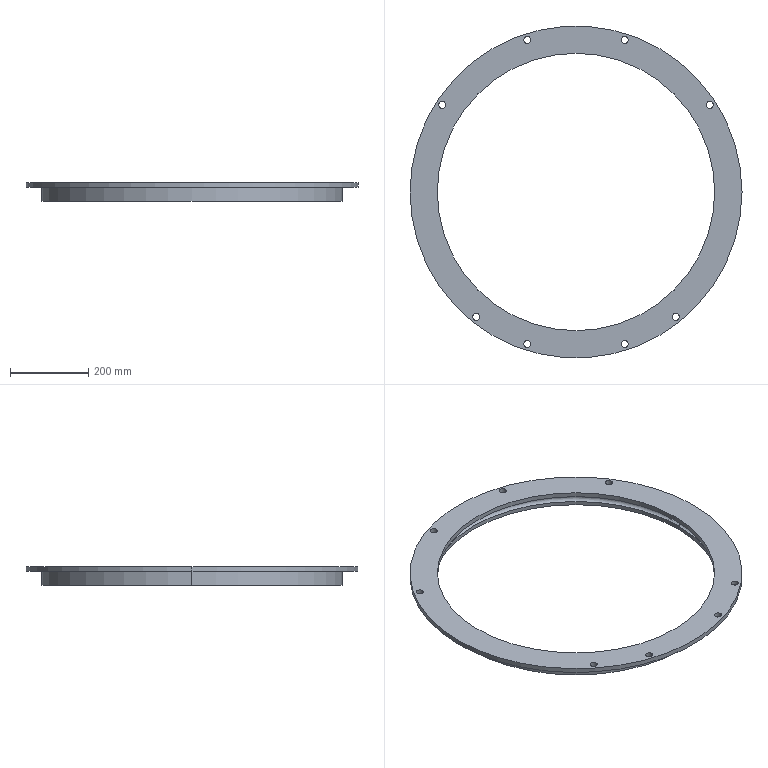Part | SolidWorks | features Cut 1, Extrusion 1, HoleWzd 1, ICE 1, SweepCut 1 | 1 solid | 34 faces | box 850 x 850 x 48 mm | volume 3078442 mm3 | cylinder 28 | plane 4 | torus 2 | commonest cylinder face diameters 18 x16 740 x4 9 x2 710 x2 770 x2 850 x2
STEP:
#1=CARTESIAN_POINT('',(116.,389.43,12.));
#2=VERTEX_POINT('',#1);
#3=CARTESIAN_POINT('',(134.,389.43,12.));
#4=VERTEX_POINT('',#3);
#5=CARTESIAN_POINT('',(125.,389.43,12.));
#6=DIRECTION('',(0.,0.,1.));
#7=DIRECTION('',(1.,0.,0.));
#8=AXIS2_PLACEMENT_3D('',#5,#6,#7);
#9=CIRCLE('',#8,9.);
#10=EDGE_CURVE('',#2,#4,#9,.T.);
#11=ORIENTED_EDGE('',*,*,#10,.T.);
#12=CARTESIAN_POINT('',(134.,389.43,0.));
#13=VERTEX_POINT('',#12);
#14=CARTESIAN_POINT('',(134.,389.43,15.));
#15=DIRECTION('',(0.,0.,-1.));
#16=VECTOR('',#15,1000.);
#17=LINE('',#14,#16);
#18=EDGE_CURVE('',#4,#13,#17,.T.);
#19=ORIENTED_EDGE('',*,*,#18,.T.);
#20=CARTESIAN_POINT('',(116.,389.43,0.));
#21=VERTEX_POINT('',#20);
#22=CARTESIAN_POINT('',(125.,389.43,0.));
#23=DIRECTION('',(0.,0.,-1.));
#24=DIRECTION('',(-1.,0.,0.));
#25=AXIS2_PLACEMENT_3D('',#22,#23,#24);
#26=CIRCLE('',#25,9.);
#27=EDGE_CURVE('',#13,#21,#26,.T.);
#28=ORIENTED_EDGE('',*,*,#27,.T.);
#29=CARTESIAN_POINT('',(116.,389.43,15.));
#30=DIRECTION('',(0.,0.,-1.));
#31=VECTOR('',#30,1000.);
#32=LINE('',#29,#31);
#33=EDGE_CURVE('',#2,#21,#32,.T.);
#34=ORIENTED_EDGE('',*,*,#33,.F.);
#35=EDGE_LOOP('',(#11,#19,#28,#34));
#36=FACE_OUTER_BOUND('',#35,.T.);
#37=CARTESIAN_POINT('',(125.,389.43,15.));
#38=DIRECTION('',(0.,0.,-1.));
#39=DIRECTION('',(-1.,0.,0.));
#40=AXIS2_PLACEMENT_3D('',#37,#38,#39);
#41=CYLINDRICAL_SURFACE('',#40,9.);
#42=ADVANCED_FACE('',(#36),#41,.F.);
#43=CARTESIAN_POINT('',(-264.409,-319.448,12.));
#44=VERTEX_POINT('',#43);
#45=CARTESIAN_POINT('',(-246.409,-319.448,12.));
#46=VERTEX_POINT('',#45);
#47=CARTESIAN_POINT('',(-255.409,-319.448,12.));
#48=DIRECTION('',(0.,0.,1.));
#49=DIRECTION('',(1.,0.,0.));
#50=AXIS2_PLACEMENT_3D('',#47,#48,#49);
#51=CIRCLE('',#50,9.);
#52=EDGE_CURVE('',#44,#46,#51,.T.);
#53=ORIENTED_EDGE('',*,*,#52,.T.);
#54=CARTESIAN_POINT('',(-246.409,-319.448,0.));
#55=VERTEX_POINT('',#54);
#56=CARTESIAN_POINT('',(-246.409,-319.448,15.));
#57=DIRECTION('',(0.,0.,-1.));
#58=VECTOR('',#57,1000.);
#59=LINE('',#56,#58);
#60=EDGE_CURVE('',#46,#55,#59,.T.);
#61=ORIENTED_EDGE('',*,*,#60,.T.);
#62=CARTESIAN_POINT('',(-264.409,-319.448,0.));
#63=VERTEX_POINT('',#62);
#64=CARTESIAN_POINT('',(-255.409,-319.448,0.));
#65=DIRECTION('',(0.,0.,-1.));
#66=DIRECTION('',(-1.,0.,0.));
#67=AXIS2_PLACEMENT_3D('',#64,#65,#66);
#68=CIRCLE('',#67,9.);
#69=EDGE_CURVE('',#55,#63,#68,.T.);
#70=ORIENTED_EDGE('',*,*,#69,.T.);
#71=CARTESIAN_POINT('',(-264.409,-319.448,15.));
#72=DIRECTION('',(0.,0.,-1.));
#73=VECTOR('',#72,1000.);
#74=LINE('',#71,#73);
#75=EDGE_CURVE('',#44,#63,#74,.T.);
#76=ORIENTED_EDGE('',*,*,#75,.F.);
#77=EDGE_LOOP('',(#53,#61,#70,#76));
#78=FACE_OUTER_BOUND('',#77,.T.);
#79=CARTESIAN_POINT('',(-255.409,-319.448,15.));
#80=DIRECTION('',(0.,0.,-1.));
#81=DIRECTION('',(-1.,0.,0.));
#82=AXIS2_PLACEMENT_3D('',#79,#80,#81);
#83=CYLINDRICAL_SURFACE('',#82,9.);
#84=ADVANCED_FACE('',(#78),#83,.F.);
#85=CARTESIAN_POINT('',(246.409,-319.448,12.));
#86=VERTEX_POINT('',#85);
#87=CARTESIAN_POINT('',(264.409,-319.448,12.));
#88=VERTEX_POINT('',#87);
#89=CARTESIAN_POINT('',(255.409,-319.448,12.));
#90=DIRECTION('',(0.,0.,1.));
#91=DIRECTION('',(1.,0.,0.));
#92=AXIS2_PLACEMENT_3D('',#89,#90,#91);
#93=CIRCLE('',#92,9.);
#94=EDGE_CURVE('',#86,#88,#93,.T.);
#95=ORIENTED_EDGE('',*,*,#94,.T.);
#96=CARTESIAN_POINT('',(264.409,-319.448,0.));
#97=VERTEX_POINT('',#96);
#98=CARTESIAN_POINT('',(264.409,-319.448,15.));
#99=DIRECTION('',(0.,0.,-1.));
#100=VECTOR('',#99,1000.);
#101=LINE('',#98,#100);
#102=EDGE_CURVE('',#88,#97,#101,.T.);
#103=ORIENTED_EDGE('',*,*,#102,.T.);
#104=CARTESIAN_POINT('',(246.409,-319.448,0.));
#105=VERTEX_POINT('',#104);
#106=CARTESIAN_POINT('',(255.409,-319.448,0.));
#107=DIRECTION('',(0.,0.,-1.));
#108=DIRECTION('',(-1.,0.,0.));
#109=AXIS2_PLACEMENT_3D('',#106,#107,#108);
#110=CIRCLE('',#109,9.);
#111=EDGE_CURVE('',#97,#105,#110,.T.);
#112=ORIENTED_EDGE('',*,*,#111,.T.);
#113=CARTESIAN_POINT('',(246.409,-319.448,15.));
#114=DIRECTION('',(0.,0.,-1.));
#115=VECTOR('',#114,1000.);
#116=LINE('',#113,#115);
#117=EDGE_CURVE('',#86,#105,#116,.T.);
#118=ORIENTED_EDGE('',*,*,#117,.F.);
#119=EDGE_LOOP('',(#95,#103,#112,#118));
#120=FACE_OUTER_BOUND('',#119,.T.);
#121=CARTESIAN_POINT('',(255.409,-319.448,15.));
#122=DIRECTION('',(0.,0.,-1.));
#123=DIRECTION('',(-1.,0.,0.));
#124=AXIS2_PLACEMENT_3D('',#121,#122,#123);
#125=CYLINDRICAL_SURFACE('',#124,9.);
#126=ADVANCED_FACE('',(#120),#125,.F.);
#127=CARTESIAN_POINT('',(-134.,-389.43,12.));
#128=VERTEX_POINT('',#127);
#129=CARTESIAN_POINT('',(-116.,-389.43,12.));
#130=VERTEX_POINT('',#129);
#131=CARTESIAN_POINT('',(-125.,-389.43,12.));
#132=DIRECTION('',(0.,0.,1.));
#133=DIRECTION('',(1.,0.,0.));
#134=AXIS2_PLACEMENT_3D('',#131,#132,#133);
#135=CIRCLE('',#134,9.);
#136=EDGE_CURVE('',#128,#130,#135,.T.);
#137=ORIENTED_EDGE('',*,*,#136,.T.);
#138=CARTESIAN_POINT('',(-116.,-389.43,0.));
#139=VERTEX_POINT('',#138);
#140=CARTESIAN_POINT('',(-116.,-389.43,15.));
#141=DIRECTION('',(0.,0.,-1.));
#142=VECTOR('',#141,1000.);
#143=LINE('',#140,#142);
#144=EDGE_CURVE('',#130,#139,#143,.T.);
#145=ORIENTED_EDGE('',*,*,#144,.T.);
#146=CARTESIAN_POINT('',(-134.,-389.43,0.));
#147=VERTEX_POINT('',#146);
#148=CARTESIAN_POINT('',(-125.,-389.43,0.));
#149=DIRECTION('',(0.,0.,-1.));
#150=DIRECTION('',(-1.,0.,0.));
#151=AXIS2_PLACEMENT_3D('',#148,#149,#150);
#152=CIRCLE('',#151,9.);
#153=EDGE_CURVE('',#139,#147,#152,.T.);
#154=ORIENTED_EDGE('',*,*,#153,.T.);
#155=CARTESIAN_POINT('',(-134.,-389.43,15.));
#156=DIRECTION('',(0.,0.,-1.));
#157=VECTOR('',#156,1000.);
#158=LINE('',#155,#157);
#159=EDGE_CURVE('',#128,#147,#158,.T.);
#160=ORIENTED_EDGE('',*,*,#159,.F.);
#161=EDGE_LOOP('',(#137,#145,#154,#160));
#162=FACE_OUTER_BOUND('',#161,.T.);
#163=CARTESIAN_POINT('',(-125.,-389.43,15.));
#164=DIRECTION('',(0.,0.,-1.));
#165=DIRECTION('',(-1.,0.,0.));
#166=AXIS2_PLACEMENT_3D('',#163,#164,#165);
#167=CYLINDRICAL_SURFACE('',#166,9.);
#168=ADVANCED_FACE('',(#162),#167,.F.);
#169=CARTESIAN_POINT('',(-134.,389.43,12.));
#170=VERTEX_POINT('',#169);
#171=CARTESIAN_POINT('',(-116.,389.43,12.));
#172=VERTEX_POINT('',#171);
#173=CARTESIAN_POINT('',(-125.,389.43,12.));
#174=DIRECTION('',(0.,0.,1.));
#175=DIRECTION('',(1.,0.,0.));
#176=AXIS2_PLACEMENT_3D('',#173,#174,#175);
#177=CIRCLE('',#176,9.);
#178=EDGE_CURVE('',#170,#172,#177,.T.);
#179=ORIENTED_EDGE('',*,*,#178,.T.);
#180=CARTESIAN_POINT('',(-116.,389.43,0.));
#181=VERTEX_POINT('',#180);
#182=CARTESIAN_POINT('',(-116.,389.43,15.));
#183=DIRECTION('',(0.,0.,-1.));
#184=VECTOR('',#183,1000.);
#185=LINE('',#182,#184);
#186=EDGE_CURVE('',#172,#181,#185,.T.);
#187=ORIENTED_EDGE('',*,*,#186,.T.);
#188=CARTESIAN_POINT('',(-134.,389.43,0.));
#189=VERTEX_POINT('',#188);
#190=CARTESIAN_POINT('',(-125.,389.43,0.));
#191=DIRECTION('',(0.,0.,-1.));
#192=DIRECTION('',(-1.,0.,0.));
#193=AXIS2_PLACEMENT_3D('',#190,#191,#192);
#194=CIRCLE('',#193,9.);
#195=EDGE_CURVE('',#181,#189,#194,.T.);
#196=ORIENTED_EDGE('',*,*,#195,.T.);
#197=CARTESIAN_POINT('',(-134.,389.43,15.));
#198=DIRECTION('',(0.,0.,-1.));
#199=VECTOR('',#198,1000.);
#200=LINE('',#197,#199);
#201=EDGE_CURVE('',#170,#189,#200,.T.);
#202=ORIENTED_EDGE('',*,*,#201,.F.);
#203=EDGE_LOOP('',(#179,#187,#196,#202));
#204=FACE_OUTER_BOUND('',#203,.T.);
#205=CARTESIAN_POINT('',(-125.,389.43,15.));
#206=DIRECTION('',(0.,0.,-1.));
#207=DIRECTION('',(-1.,0.,0.));
#208=AXIS2_PLACEMENT_3D('',#205,#206,#207);
#209=CYLINDRICAL_SURFACE('',#208,9.);
#210=ADVANCED_FACE('',(#204),#209,.F.);
#211=CARTESIAN_POINT('',(-351.768,223.139,12.));
#212=VERTEX_POINT('',#211);
#213=CARTESIAN_POINT('',(-333.768,223.139,12.));
#214=VERTEX_POINT('',#213);
#215=CARTESIAN_POINT('',(-342.768,223.139,12.));
#216=DIRECTION('',(0.,0.,1.));
#217=DIRECTION('',(1.,0.,0.));
#218=AXIS2_PLACEMENT_3D('',#215,#216,#217);
#219=CIRCLE('',#218,9.);
#220=EDGE_CURVE('',#212,#214,#219,.T.);
#221=ORIENTED_EDGE('',*,*,#220,.T.);
#222=CARTESIAN_POINT('',(-333.768,223.139,0.));
#223=VERTEX_POINT('',#222);
#224=CARTESIAN_POINT('',(-333.768,223.139,15.));
#225=DIRECTION('',(0.,0.,-1.));
#226=VECTOR('',#225,1000.);
#227=LINE('',#224,#226);
#228=EDGE_CURVE('',#214,#223,#227,.T.);
#229=ORIENTED_EDGE('',*,*,#228,.T.);
#230=CARTESIAN_POINT('',(-351.768,223.139,0.));
#231=VERTEX_POINT('',#230);
#232=CARTESIAN_POINT('',(-342.768,223.139,0.));
#233=DIRECTION('',(0.,0.,-1.));
#234=DIRECTION('',(-1.,0.,0.));
#235=AXIS2_PLACEMENT_3D('',#232,#233,#234);
#236=CIRCLE('',#235,9.);
#237=EDGE_CURVE('',#223,#231,#236,.T.);
#238=ORIENTED_EDGE('',*,*,#237,.T.);
#239=CARTESIAN_POINT('',(-351.768,223.139,15.));
#240=DIRECTION('',(0.,0.,-1.));
#241=VECTOR('',#240,1000.);
#242=LINE('',#239,#241);
#243=EDGE_CURVE('',#212,#231,#242,.T.);
#244=ORIENTED_EDGE('',*,*,#243,.F.);
#245=EDGE_LOOP('',(#221,#229,#238,#244));
#246=FACE_OUTER_BOUND('',#245,.T.);
#247=CARTESIAN_POINT('',(-342.768,223.139,15.));
#248=DIRECTION('',(0.,0.,-1.));
#249=DIRECTION('',(-1.,0.,0.));
#250=AXIS2_PLACEMENT_3D('',#247,#248,#249);
#251=CYLINDRICAL_SURFACE('',#250,9.);
#252=ADVANCED_FACE('',(#246),#251,.F.);
#253=CARTESIAN_POINT('',(333.768,223.139,12.));
#254=VERTEX_POINT('',#253);
#255=CARTESIAN_POINT('',(351.768,223.139,12.));
#256=VERTEX_POINT('',#255);
#257=CARTESIAN_POINT('',(342.768,223.139,12.));
#258=DIRECTION('',(0.,0.,1.));
#259=DIRECTION('',(1.,0.,0.));
#260=AXIS2_PLACEMENT_3D('',#257,#258,#259);
#261=CIRCLE('',#260,9.);
#262=EDGE_CURVE('',#254,#256,#261,.T.);
#263=ORIENTED_EDGE('',*,*,#262,.T.);
#264=CARTESIAN_POINT('',(351.768,223.139,0.));
#265=VERTEX_POINT('',#264);
#266=CARTESIAN_POINT('',(351.768,223.139,15.));
#267=DIRECTION('',(0.,0.,-1.));
#268=VECTOR('',#267,1000.);
#269=LINE('',#266,#268);
#270=EDGE_CURVE('',#256,#265,#269,.T.);
#271=ORIENTED_EDGE('',*,*,#270,.T.);
#272=CARTESIAN_POINT('',(333.768,223.139,0.));
#273=VERTEX_POINT('',#272);
#274=CARTESIAN_POINT('',(342.768,223.139,0.));
#275=DIRECTION('',(0.,0.,-1.));
#276=DIRECTION('',(-1.,0.,0.));
#277=AXIS2_PLACEMENT_3D('',#274,#275,#276);
#278=CIRCLE('',#277,9.);
#279=EDGE_CURVE('',#265,#273,#278,.T.);
#280=ORIENTED_EDGE('',*,*,#279,.T.);
#281=CARTESIAN_POINT('',(333.768,223.139,15.));
#282=DIRECTION('',(0.,0.,-1.));
#283=VECTOR('',#282,1000.);
#284=LINE('',#281,#283);
#285=EDGE_CURVE('',#254,#273,#284,.T.);
#286=ORIENTED_EDGE('',*,*,#285,.F.);
#287=EDGE_LOOP('',(#263,#271,#280,#286));
#288=FACE_OUTER_BOUND('',#287,.T.);
#289=CARTESIAN_POINT('',(342.768,223.139,15.));
#290=DIRECTION('',(0.,0.,-1.));
#291=DIRECTION('',(-1.,0.,0.));
#292=AXIS2_PLACEMENT_3D('',#289,#290,#291);
#293=CYLINDRICAL_SURFACE('',#292,9.);
#294=ADVANCED_FACE('',(#288),#293,.F.);
#295=CARTESIAN_POINT('',(116.,-389.43,12.));
#296=VERTEX_POINT('',#295);
#297=CARTESIAN_POINT('',(134.,-389.43,12.));
#298=VERTEX_POINT('',#297);
#299=CARTESIAN_POINT('',(125.,-389.43,12.));
#300=DIRECTION('',(0.,0.,1.));
#301=DIRECTION('',(1.,0.,0.));
#302=AXIS2_PLACEMENT_3D('',#299,#300,#301);
#303=CIRCLE('',#302,9.);
#304=EDGE_CURVE('',#296,#298,#303,.T.);
#305=ORIENTED_EDGE('',*,*,#304,.T.);
#306=CARTESIAN_POINT('',(134.,-389.43,0.));
#307=VERTEX_POINT('',#306);
#308=CARTESIAN_POINT('',(134.,-389.43,15.));
#309=DIRECTION('',(0.,0.,-1.));
#310=VECTOR('',#309,1000.);
#311=LINE('',#308,#310);
#312=EDGE_CURVE('',#298,#307,#311,.T.);
#313=ORIENTED_EDGE('',*,*,#312,.T.);
#314=CARTESIAN_POINT('',(116.,-389.43,0.));
#315=VERTEX_POINT('',#314);
#316=CARTESIAN_POINT('',(125.,-389.43,0.));
#317=DIRECTION('',(0.,0.,-1.));
#318=DIRECTION('',(-1.,0.,0.));
#319=AXIS2_PLACEMENT_3D('',#316,#317,#318);
#320=CIRCLE('',#319,9.);
#321=EDGE_CURVE('',#307,#315,#320,.T.);
#322=ORIENTED_EDGE('',*,*,#321,.T.);
#323=CARTESIAN_POINT('',(116.,-389.43,15.));
#324=DIRECTION('',(0.,0.,-1.));
#325=VECTOR('',#324,1000.);
#326=LINE('',#323,#325);
#327=EDGE_CURVE('',#296,#315,#326,.T.);
#328=ORIENTED_EDGE('',*,*,#327,.F.);
#329=EDGE_LOOP('',(#305,#313,#322,#328));
#330=FACE_OUTER_BOUND('',#329,.T.);
#331=CARTESIAN_POINT('',(125.,-389.43,15.));
#332=DIRECTION('',(0.,0.,-1.));
#333=DIRECTION('',(-1.,0.,0.));
#334=AXIS2_PLACEMENT_3D('',#331,#332,#333);
#335=CYLINDRICAL_SURFACE('',#334,9.);
#336=ADVANCED_FACE('',(#330),#335,.F.);
#337=CARTESIAN_POINT('',(385.,0.,-22.5));
#338=VERTEX_POINT('',#337);
#339=CARTESIAN_POINT('',(385.,0.,-13.5));
#340=VERTEX_POINT('',#339);
#341=CARTESIAN_POINT('',(385.,0.,-22.5));
#342=CARTESIAN_POINT('',(385.,-0.2973,-22.5));
#343=CARTESIAN_POINT('',(385.,-0.5897,-22.471));
#344=CARTESIAN_POINT('',(384.998,-1.165,-22.356));
#345=CARTESIAN_POINT('',(384.997,-1.451,-22.27));
#346=CARTESIAN_POINT('',(384.995,-1.996,-22.044));
#347=CARTESIAN_POINT('',(384.993,-2.254,-21.906));
#348=CARTESIAN_POINT('',(384.99,-2.743,-21.579));
#349=CARTESIAN_POINT('',(384.989,-2.975,-21.389));
#350=CARTESIAN_POINT('',(384.985,-3.39,-20.974));
#351=CARTESIAN_POINT('',(384.983,-3.576,-20.747));
#352=CARTESIAN_POINT('',(384.98,-3.905,-20.255));
#353=CARTESIAN_POINT('',(384.979,-4.045,-19.993));
#354=CARTESIAN_POINT('',(384.976,-4.269,-19.452));
#355=CARTESIAN_POINT('',(384.975,-4.356,-19.168));
#356=CARTESIAN_POINT('',(384.974,-4.471,-18.587));
#357=CARTESIAN_POINT('',(384.974,-4.5,-18.295));
#358=CARTESIAN_POINT('',(384.974,-4.5,-17.708));
#359=CARTESIAN_POINT('',(384.974,-4.471,-17.41));
#360=CARTESIAN_POINT('',(384.975,-4.356,-16.833));
#361=CARTESIAN_POINT('',(384.976,-4.271,-16.552));
#362=CARTESIAN_POINT('',(384.979,-4.046,-16.007));
#363=CARTESIAN_POINT('',(384.98,-3.905,-15.744));
#364=CARTESIAN_POINT('',(384.983,-3.579,-15.256));
#365=CARTESIAN_POINT('',(384.985,-3.393,-15.029));
#366=CARTESIAN_POINT('',(384.989,-2.973,-14.609));
#367=CARTESIAN_POINT('',(384.99,-2.745,-14.422));
#368=CARTESIAN_POINT('',(384.993,-2.258,-14.096));
#369=CARTESIAN_POINT('',(384.995,-1.995,-13.955));
#370=CARTESIAN_POINT('',(384.997,-1.449,-13.729));
#371=CARTESIAN_POINT('',(384.998,-1.169,-13.644));
#372=CARTESIAN_POINT('',(385.,-0.592,-13.529));
#373=CARTESIAN_POINT('',(385.,-0.2937,-13.5));
#374=CARTESIAN_POINT('',(385.,0.,-13.5));
#375=B_SPLINE_CURVE_WITH_KNOTS('',3,(#341,#342,#343,#344,#345,#346,#347,#348,#349,#350,#351,#352,#353,#354,#355,#356,#357,#358,#359,#360,#361,#362,#363,#364,#365,#366,#367,#368,#369,#370,#371,#372,#373,#374),.UNSPECIFIED.,.F.,.F.,(4,2,2,2,2,2,2,2,2,2,2,2,2,2,2,2,4),(0.,0.0008793,0.001759,0.002638,0.003517,0.004397,0.005276,0.006155,0.007035,0.007914,0.008793,0.009673,0.01055,0.01143,0.01231,0.01319,0.01407),.UNSPECIFIED.);
#376=EDGE_CURVE('',#338,#340,#375,.T.);
#377=ORIENTED_EDGE('',*,*,#376,.F.);
#378=CARTESIAN_POINT('',(376.614,0.,-22.5));
#379=VERTEX_POINT('',#378);
#380=CARTESIAN_POINT('',(0.,0.,-22.5));
#381=DIRECTION('',(-1.,0.,0.));
#382=VECTOR('',#381,1000.);
#383=LINE('',#380,#382);
#384=EDGE_CURVE('',#338,#379,#383,.T.);
#385=ORIENTED_EDGE('',*,*,#384,.T.);
#386=CARTESIAN_POINT('',(376.614,0.,-13.5));
#387=VERTEX_POINT('',#386);
#388=CARTESIAN_POINT('',(376.614,0.,-13.5));
#389=CARTESIAN_POINT('',(376.614,-0.3013,-13.5));
#390=CARTESIAN_POINT('',(376.635,-0.5988,-13.53));
#391=CARTESIAN_POINT('',(376.712,-1.187,-13.649));
#392=CARTESIAN_POINT('',(376.768,-1.472,-13.738));
#393=CARTESIAN_POINT('',(376.904,-2.013,-13.965));
#394=CARTESIAN_POINT('',(376.984,-2.273,-14.105));
#395=CARTESIAN_POINT('',(377.151,-2.753,-14.428));
#396=CARTESIAN_POINT('',(377.238,-2.975,-14.611));
#397=CARTESIAN_POINT('',(377.413,-3.384,-15.02));
#398=CARTESIAN_POINT('',(377.498,-3.57,-15.245));
#399=CARTESIAN_POINT('',(377.654,-3.893,-15.724));
#400=CARTESIAN_POINT('',(377.724,-4.032,-15.98));
#401=CARTESIAN_POINT('',(377.845,-4.264,-16.53));
#402=CARTESIAN_POINT('',(377.892,-4.351,-16.813));
#403=CARTESIAN_POINT('',(377.94,-4.439,-17.25));
#404=CARTESIAN_POINT('',(377.952,-4.462,-17.397));
#405=CARTESIAN_POINT('',(377.969,-4.492,-17.697));
#406=CARTESIAN_POINT('',(377.973,-4.5,-17.85));
#407=CARTESIAN_POINT('',(377.973,-4.5,-18.303));
#408=CARTESIAN_POINT('',(377.956,-4.47,-18.6));
#409=CARTESIAN_POINT('',(377.908,-4.38,-19.041));
#410=CARTESIAN_POINT('',(377.888,-4.343,-19.188));
#411=CARTESIAN_POINT('',(377.84,-4.255,-19.474));
#412=CARTESIAN_POINT('',(377.814,-4.204,-19.613));
#413=CARTESIAN_POINT('',(377.724,-4.032,-20.02));
#414=CARTESIAN_POINT('',(377.652,-3.89,-20.28));
#415=CARTESIAN_POINT('',(377.495,-3.563,-20.764));
#416=CARTESIAN_POINT('',(377.41,-3.379,-20.986));
#417=CARTESIAN_POINT('',(377.236,-2.969,-21.394));
#418=CARTESIAN_POINT('',(377.147,-2.744,-21.578));
#419=CARTESIAN_POINT('',(376.981,-2.266,-21.899));
#420=CARTESIAN_POINT('',(376.903,-2.011,-22.037));
#421=CARTESIAN_POINT('',(376.767,-1.466,-22.265));
#422=CARTESIAN_POINT('',(376.712,-1.185,-22.351));
#423=CARTESIAN_POINT('',(376.654,-0.7496,-22.44));
#424=CARTESIAN_POINT('',(376.64,-0.6023,-22.462));
#425=CARTESIAN_POINT('',(376.62,-0.3029,-22.492));
#426=CARTESIAN_POINT('',(376.614,-0.1504,-22.5));
#427=CARTESIAN_POINT('',(376.614,0.,-22.5));
#428=B_SPLINE_CURVE_WITH_KNOTS('',3,(#388,#389,#390,#391,#392,#393,#394,#395,#396,#397,#398,#399,#400,#401,#402,#403,#404,#405,#406,#407,#408,#409,#410,#411,#412,#413,#414,#415,#416,#417,#418,#419,#420,#421,#422,#423,#424,#425,#426,#427),.UNSPECIFIED.,.F.,.F.,(4,2,2,2,2,2,2,2,2,2,2,2,2,2,2,2,2,2,2,4),(0.01771,0.01861,0.01951,0.0204,0.0213,0.0222,0.0231,0.02399,0.02444,0.02489,0.02579,0.02624,0.02669,0.02759,0.02848,0.02938,0.03028,0.03118,0.03163,0.03208),.UNSPECIFIED.);
#429=EDGE_CURVE('',#387,#379,#428,.T.);
#430=ORIENTED_EDGE('',*,*,#429,.F.);
#431=CARTESIAN_POINT('',(0.,0.,-13.5));
#432=DIRECTION('',(-1.,0.,0.));
#433=VECTOR('',#432,1000.);
#434=LINE('',#431,#433);
#435=EDGE_CURVE('',#340,#387,#434,.T.);
#436=ORIENTED_EDGE('',*,*,#435,.F.);
#437=EDGE_LOOP('',(#377,#385,#430,#436));
#438=FACE_OUTER_BOUND('',#437,.T.);
#439=CARTESIAN_POINT('',(0.,0.,-18.));
#440=DIRECTION('',(-1.,0.,0.));
#441=DIRECTION('',(0.,0.,1.));
#442=AXIS2_PLACEMENT_3D('',#439,#440,#441);
#443=CYLINDRICAL_SURFACE('',#442,4.5);
#444=ADVANCED_FACE('',(#438),#443,.F.);
#445=CARTESIAN_POINT('',(370.,0.,-26.));
#446=VERTEX_POINT('',#445);
#447=CARTESIAN_POINT('',(-370.,0.,-26.));
#448=VERTEX_POINT('',#447);
#449=CARTESIAN_POINT('',(0.,0.,-26.));
#450=DIRECTION('',(0.,0.,-1.));
#451=DIRECTION('',(1.,0.,0.));
#452=AXIS2_PLACEMENT_3D('',#449,#450,#451);
#453=CIRCLE('',#452,370.);
#454=EDGE_CURVE('',#446,#448,#453,.T.);
#455=ORIENTED_EDGE('',*,*,#454,.T.);
#456=CARTESIAN_POINT('',(-370.,0.,-10.));
#457=VERTEX_POINT('',#456);
#458=CARTESIAN_POINT('',(-370.,0.,-18.));
#459=DIRECTION('',(0.,1.,0.));
#460=DIRECTION('',(-1.,0.,0.));
#461=AXIS2_PLACEMENT_3D('',#458,#459,#460);
#462=CIRCLE('',#461,8.);
#463=EDGE_CURVE('',#448,#457,#462,.T.);
#464=ORIENTED_EDGE('',*,*,#463,.T.);
#465=CARTESIAN_POINT('',(370.,0.,-10.));
#466=VERTEX_POINT('',#465);
#467=CARTESIAN_POINT('',(0.,0.,-10.));
#468=DIRECTION('',(0.,0.,1.));
#469=DIRECTION('',(-1.,0.,0.));
#470=AXIS2_PLACEMENT_3D('',#467,#468,#469);
#471=CIRCLE('',#470,370.);
#472=EDGE_CURVE('',#457,#466,#471,.T.);
#473=ORIENTED_EDGE('',*,*,#472,.T.);
#474=CARTESIAN_POINT('',(370.,0.,-18.));
#475=DIRECTION('',(0.,-1.,0.));
#476=DIRECTION('',(0.,0.,-1.));
#477=AXIS2_PLACEMENT_3D('',#474,#475,#476);
#478=CIRCLE('',#477,8.);
#479=EDGE_CURVE('',#387,#466,#478,.T.);
#480=ORIENTED_EDGE('',*,*,#479,.F.);
#481=ORIENTED_EDGE('',*,*,#429,.T.);
#482=CARTESIAN_POINT('',(370.,0.,-18.));
#483=DIRECTION('',(0.,-1.,0.));
#484=DIRECTION('',(0.,0.,-1.));
#485=AXIS2_PLACEMENT_3D('',#482,#483,#484);
#486=CIRCLE('',#485,8.);
#487=EDGE_CURVE('',#446,#379,#486,.T.);
#488=ORIENTED_EDGE('',*,*,#487,.F.);
#489=EDGE_LOOP('',(#455,#464,#473,#480,#481,#488));
#490=FACE_OUTER_BOUND('',#489,.T.);
#491=CARTESIAN_POINT('',(0.,0.,-18.));
#492=DIRECTION('',(0.,0.,1.));
#493=DIRECTION('',(1.,0.,0.));
#494=AXIS2_PLACEMENT_3D('',#491,#492,#493);
#495=TOROIDAL_SURFACE('',#494,370.,8.);
#496=ADVANCED_FACE('',(#490),#495,.F.);
#497=CARTESIAN_POINT('',(370.,0.,-36.));
#498=VERTEX_POINT('',#497);
#499=CARTESIAN_POINT('',(-370.,0.,-36.));
#500=VERTEX_POINT('',#499);
#501=CARTESIAN_POINT('',(0.,0.,-36.));
#502=DIRECTION('',(0.,0.,-1.));
#503=DIRECTION('',(-1.,0.,0.));
#504=AXIS2_PLACEMENT_3D('',#501,#502,#503);
#505=CIRCLE('',#504,370.);
#506=EDGE_CURVE('',#498,#500,#505,.T.);
#507=ORIENTED_EDGE('',*,*,#506,.T.);
#508=CARTESIAN_POINT('',(-370.,0.,-36.));
#509=DIRECTION('',(0.,0.,1.));
#510=VECTOR('',#509,1000.);
#511=LINE('',#508,#510);
#512=EDGE_CURVE('',#500,#448,#511,.T.);
#513=ORIENTED_EDGE('',*,*,#512,.T.);
#514=ORIENTED_EDGE('',*,*,#454,.F.);
#515=CARTESIAN_POINT('',(370.,0.,-36.));
#516=DIRECTION('',(0.,0.,1.));
#517=VECTOR('',#516,1000.);
#518=LINE('',#515,#517);
#519=EDGE_CURVE('',#498,#446,#518,.T.);
#520=ORIENTED_EDGE('',*,*,#519,.F.);
#521=EDGE_LOOP('',(#507,#513,#514,#520));
#522=FACE_OUTER_BOUND('',#521,.T.);
#523=CARTESIAN_POINT('',(0.,0.,-36.));
#524=DIRECTION('',(0.,0.,1.));
#525=DIRECTION('',(1.,0.,0.));
#526=AXIS2_PLACEMENT_3D('',#523,#524,#525);
#527=CYLINDRICAL_SURFACE('',#526,370.);
#528=ADVANCED_FACE('',(#522),#527,.F.);
#529=CARTESIAN_POINT('',(-385.,0.,-36.));
#530=VERTEX_POINT('',#529);
#531=CARTESIAN_POINT('',(385.,0.,-36.));
#532=VERTEX_POINT('',#531);
#533=CARTESIAN_POINT('',(0.,0.,-36.));
#534=DIRECTION('',(0.,0.,-1.));
#535=DIRECTION('',(-1.,0.,0.));
#536=AXIS2_PLACEMENT_3D('',#533,#534,#535);
#537=CIRCLE('',#536,385.);
#538=EDGE_CURVE('',#530,#532,#537,.T.);
#539=ORIENTED_EDGE('',*,*,#538,.F.);
#540=CARTESIAN_POINT('',(-385.,0.,0.));
#541=VERTEX_POINT('',#540);
#542=CARTESIAN_POINT('',(-385.,0.,-36.));
#543=DIRECTION('',(0.,0.,1.));
#544=VECTOR('',#543,1000.);
#545=LINE('',#542,#544);
#546=EDGE_CURVE('',#530,#541,#545,.T.);
#547=ORIENTED_EDGE('',*,*,#546,.T.);
#548=CARTESIAN_POINT('',(385.,0.,0.));
#549=VERTEX_POINT('',#548);
#550=CARTESIAN_POINT('',(0.,0.,0.));
#551=DIRECTION('',(0.,0.,-1.));
#552=DIRECTION('',(1.,0.,0.));
#553=AXIS2_PLACEMENT_3D('',#550,#551,#552);
#554=CIRCLE('',#553,385.);
#555=EDGE_CURVE('',#541,#549,#554,.T.);
#556=ORIENTED_EDGE('',*,*,#555,.T.);
#557=CARTESIAN_POINT('',(385.,0.,-36.));
#558=DIRECTION('',(0.,0.,1.));
#559=VECTOR('',#558,1000.);
#560=LINE('',#557,#559);
#561=EDGE_CURVE('',#340,#549,#560,.T.);
#562=ORIENTED_EDGE('',*,*,#561,.F.);
#563=CARTESIAN_POINT('',(385.,0.,-13.5));
#564=CARTESIAN_POINT('',(385.,0.2936,-13.5));
#565=CARTESIAN_POINT('',(385.,0.5855,-13.528));
#566=CARTESIAN_POINT('',(384.998,1.165,-13.643));
#567=CARTESIAN_POINT('',(384.997,1.45,-13.73));
#568=CARTESIAN_POINT('',(384.995,1.991,-13.954));
#569=CARTESIAN_POINT('',(384.993,2.253,-14.093));
#570=CARTESIAN_POINT('',(384.99,2.745,-14.422));
#571=CARTESIAN_POINT('',(384.989,2.972,-14.608));
#572=CARTESIAN_POINT('',(384.985,3.387,-15.023));
#573=CARTESIAN_POINT('',(384.983,3.577,-15.254));
#574=CARTESIAN_POINT('',(384.98,3.905,-15.744));
#575=CARTESIAN_POINT('',(384.979,4.043,-16.002));
#576=CARTESIAN_POINT('',(384.976,4.269,-16.546));
#577=CARTESIAN_POINT('',(384.975,4.356,-16.832));
#578=CARTESIAN_POINT('',(384.974,4.47,-17.407));
#579=CARTESIAN_POINT('',(384.974,4.5,-17.7));
#580=CARTESIAN_POINT('',(384.974,4.5,-18.293));
#581=CARTESIAN_POINT('',(384.974,4.471,-18.587));
#582=CARTESIAN_POINT('',(384.975,4.357,-19.162));
#583=CARTESIAN_POINT('',(384.976,4.271,-19.447));
#584=CARTESIAN_POINT('',(384.979,4.046,-19.993));
#585=CARTESIAN_POINT('',(384.98,3.908,-20.251));
#586=CARTESIAN_POINT('',(384.983,3.582,-20.74));
#587=CARTESIAN_POINT('',(384.985,3.392,-20.972));
#588=CARTESIAN_POINT('',(384.989,2.977,-21.388));
#589=CARTESIAN_POINT('',(384.99,2.75,-21.574));
#590=CARTESIAN_POINT('',(384.993,2.26,-21.903));
#591=CARTESIAN_POINT('',(384.995,1.997,-22.043));
#592=CARTESIAN_POINT('',(384.997,1.456,-22.268));
#593=CARTESIAN_POINT('',(384.998,1.174,-22.354));
#594=CARTESIAN_POINT('',(385.,0.5914,-22.471));
#595=CARTESIAN_POINT('',(385.,0.2973,-22.5));
#596=CARTESIAN_POINT('',(385.,0.,-22.5));
#597=B_SPLINE_CURVE_WITH_KNOTS('',3,(#563,#564,#565,#566,#567,#568,#569,#570,#571,#572,#573,#574,#575,#576,#577,#578,#579,#580,#581,#582,#583,#584,#585,#586,#587,#588,#589,#590,#591,#592,#593,#594,#595,#596),.UNSPECIFIED.,.F.,.F.,(4,2,2,2,2,2,2,2,2,2,2,2,2,2,2,2,4),(0.01407,0.01495,0.01583,0.01671,0.01759,0.01846,0.01934,0.02022,0.0211,0.02198,0.02286,0.02374,0.02462,0.0255,0.02638,0.02726,0.02814),.UNSPECIFIED.);
#598=EDGE_CURVE('',#340,#338,#597,.T.);
#599=ORIENTED_EDGE('',*,*,#598,.T.);
#600=CARTESIAN_POINT('',(385.,0.,-36.));
#601=DIRECTION('',(0.,0.,1.));
#602=VECTOR('',#601,1000.);
#603=LINE('',#600,#602);
#604=EDGE_CURVE('',#532,#338,#603,.T.);
#605=ORIENTED_EDGE('',*,*,#604,.F.);
#606=EDGE_LOOP('',(#539,#547,#556,#562,#599,#605));
#607=FACE_OUTER_BOUND('',#606,.T.);
#608=CARTESIAN_POINT('',(0.,0.,-36.));
#609=DIRECTION('',(0.,0.,1.));
#610=DIRECTION('',(1.,0.,0.));
#611=AXIS2_PLACEMENT_3D('',#608,#609,#610);
#612=CYLINDRICAL_SURFACE('',#611,385.);
#613=ADVANCED_FACE('',(#607),#612,.T.);
#614=CARTESIAN_POINT('',(-355.,0.,12.));
#615=VERTEX_POINT('',#614);
#616=CARTESIAN_POINT('',(355.,0.,12.));
#617=VERTEX_POINT('',#616);
#618=CARTESIAN_POINT('',(0.,0.,12.));
#619=DIRECTION('',(0.,0.,1.));
#620=DIRECTION('',(1.,0.,0.));
#621=AXIS2_PLACEMENT_3D('',#618,#619,#620);
#622=CIRCLE('',#621,355.);
#623=EDGE_CURVE('',#615,#617,#622,.T.);
#624=ORIENTED_EDGE('',*,*,#623,.T.);
#625=CARTESIAN_POINT('',(355.,0.,0.));
#626=VERTEX_POINT('',#625);
#627=CARTESIAN_POINT('',(355.,0.,12.));
#628=DIRECTION('',(0.,0.,-1.));
#629=VECTOR('',#628,1000.);
#630=LINE('',#627,#629);
#631=EDGE_CURVE('',#617,#626,#630,.T.);
#632=ORIENTED_EDGE('',*,*,#631,.T.);
#633=CARTESIAN_POINT('',(-355.,0.,0.));
#634=VERTEX_POINT('',#633);
#635=CARTESIAN_POINT('',(0.,0.,0.));
#636=DIRECTION('',(0.,0.,1.));
#637=DIRECTION('',(1.,0.,0.));
#638=AXIS2_PLACEMENT_3D('',#635,#636,#637);
#639=CIRCLE('',#638,355.);
#640=EDGE_CURVE('',#634,#626,#639,.T.);
#641=ORIENTED_EDGE('',*,*,#640,.F.);
#642=CARTESIAN_POINT('',(-355.,0.,12.));
#643=DIRECTION('',(0.,0.,-1.));
#644=VECTOR('',#643,1000.);
#645=LINE('',#642,#644);
#646=EDGE_CURVE('',#615,#634,#645,.T.);
#647=ORIENTED_EDGE('',*,*,#646,.F.);
#648=EDGE_LOOP('',(#624,#632,#641,#647));
#649=FACE_OUTER_BOUND('',#648,.T.);
#650=CARTESIAN_POINT('',(0.,0.,12.));
#651=DIRECTION('',(0.,0.,-1.));
#652=DIRECTION('',(-1.,0.,0.));
#653=AXIS2_PLACEMENT_3D('',#650,#651,#652);
#654=CYLINDRICAL_SURFACE('',#653,355.);
#655=ADVANCED_FACE('',(#649),#654,.F.);
#656=CARTESIAN_POINT('',(425.,0.,12.));
#657=VERTEX_POINT('',#656);
#658=CARTESIAN_POINT('',(-425.,0.,12.));
#659=VERTEX_POINT('',#658);
#660=CARTESIAN_POINT('',(0.,0.,12.));
#661=DIRECTION('',(0.,0.,1.));
#662=DIRECTION('',(1.,0.,0.));
#663=AXIS2_PLACEMENT_3D('',#660,#661,#662);
#664=CIRCLE('',#663,425.);
#665=EDGE_CURVE('',#657,#659,#664,.T.);
#666=ORIENTED_EDGE('',*,*,#665,.F.);
#667=CARTESIAN_POINT('',(425.,0.,0.));
#668=VERTEX_POINT('',#667);
#669=CARTESIAN_POINT('',(425.,0.,12.));
#670=DIRECTION('',(0.,0.,-1.));
#671=VECTOR('',#670,1000.);
#672=LINE('',#669,#671);
#673=EDGE_CURVE('',#657,#668,#672,.T.);
#674=ORIENTED_EDGE('',*,*,#673,.T.);
#675=CARTESIAN_POINT('',(-425.,0.,0.));
#676=VERTEX_POINT('',#675);
#677=CARTESIAN_POINT('',(0.,0.,0.));
#678=DIRECTION('',(0.,0.,1.));
#679=DIRECTION('',(1.,0.,0.));
#680=AXIS2_PLACEMENT_3D('',#677,#678,#679);
#681=CIRCLE('',#680,425.);
#682=EDGE_CURVE('',#668,#676,#681,.T.);
#683=ORIENTED_EDGE('',*,*,#682,.T.);
#684=CARTESIAN_POINT('',(-425.,0.,12.));
#685=DIRECTION('',(0.,0.,-1.));
#686=VECTOR('',#685,1000.);
#687=LINE('',#684,#686);
#688=EDGE_CURVE('',#659,#676,#687,.T.);
#689=ORIENTED_EDGE('',*,*,#688,.F.);
#690=EDGE_LOOP('',(#666,#674,#683,#689));
#691=FACE_OUTER_BOUND('',#690,.T.);
#692=CARTESIAN_POINT('',(0.,0.,12.));
#693=DIRECTION('',(0.,0.,-1.));
#694=DIRECTION('',(-1.,0.,0.));
#695=AXIS2_PLACEMENT_3D('',#692,#693,#694);
#696=CYLINDRICAL_SURFACE('',#695,425.);
#697=ADVANCED_FACE('',(#691),#696,.T.);
#698=ORIENTED_EDGE('',*,*,#472,.F.);
#699=CARTESIAN_POINT('',(-370.,0.,0.));
#700=VERTEX_POINT('',#699);
#701=CARTESIAN_POINT('',(-370.,0.,-36.));
#702=DIRECTION('',(0.,0.,1.));
#703=VECTOR('',#702,1000.);
#704=LINE('',#701,#703);
#705=EDGE_CURVE('',#457,#700,#704,.T.);
#706=ORIENTED_EDGE('',*,*,#705,.T.);
#707=CARTESIAN_POINT('',(370.,0.,0.));
#708=VERTEX_POINT('',#707);
#709=CARTESIAN_POINT('',(0.,0.,0.));
#710=DIRECTION('',(0.,0.,-1.));
#711=DIRECTION('',(-1.,0.,0.));
#712=AXIS2_PLACEMENT_3D('',#709,#710,#711);
#713=CIRCLE('',#712,370.);
#714=EDGE_CURVE('',#708,#700,#713,.T.);
#715=ORIENTED_EDGE('',*,*,#714,.F.);
#716=CARTESIAN_POINT('',(370.,0.,-36.));
#717=DIRECTION('',(0.,0.,1.));
#718=VECTOR('',#717,1000.);
#719=LINE('',#716,#718);
#720=EDGE_CURVE('',#466,#708,#719,.T.);
#721=ORIENTED_EDGE('',*,*,#720,.F.);
#722=EDGE_LOOP('',(#698,#706,#715,#721));
#723=FACE_OUTER_BOUND('',#722,.T.);
#724=CARTESIAN_POINT('',(0.,0.,-36.));
#725=DIRECTION('',(0.,0.,1.));
#726=DIRECTION('',(1.,0.,0.));
#727=AXIS2_PLACEMENT_3D('',#724,#725,#726);
#728=CYLINDRICAL_SURFACE('',#727,370.);
#729=ADVANCED_FACE('',(#723),#728,.F.);
#730=ORIENTED_EDGE('',*,*,#705,.F.);
#731=CARTESIAN_POINT('',(0.,0.,-10.));
#732=DIRECTION('',(0.,0.,1.));
#733=DIRECTION('',(-1.,0.,0.));
#734=AXIS2_PLACEMENT_3D('',#731,#732,#733);
#735=CIRCLE('',#734,370.);
#736=EDGE_CURVE('',#466,#457,#735,.T.);
#737=ORIENTED_EDGE('',*,*,#736,.F.);
#738=ORIENTED_EDGE('',*,*,#720,.T.);
#739=CARTESIAN_POINT('',(0.,0.,0.));
#740=DIRECTION('',(0.,0.,-1.));
#741=DIRECTION('',(-1.,0.,0.));
#742=AXIS2_PLACEMENT_3D('',#739,#740,#741);
#743=CIRCLE('',#742,370.);
#744=EDGE_CURVE('',#700,#708,#743,.T.);
#745=ORIENTED_EDGE('',*,*,#744,.F.);
#746=EDGE_LOOP('',(#730,#737,#738,#745));
#747=FACE_OUTER_BOUND('',#746,.T.);
#748=CARTESIAN_POINT('',(0.,0.,-36.));
#749=DIRECTION('',(0.,0.,1.));
#750=DIRECTION('',(1.,0.,0.));
#751=AXIS2_PLACEMENT_3D('',#748,#749,#750);
#752=CYLINDRICAL_SURFACE('',#751,370.);
#753=ADVANCED_FACE('',(#747),#752,.F.);
#754=ORIENTED_EDGE('',*,*,#640,.T.);
#755=CARTESIAN_POINT('',(0.,0.,0.));
#756=DIRECTION('',(0.,0.,1.));
#757=DIRECTION('',(1.,0.,0.));
#758=AXIS2_PLACEMENT_3D('',#755,#756,#757);
#759=CIRCLE('',#758,355.);
#760=EDGE_CURVE('',#626,#634,#759,.T.);
#761=ORIENTED_EDGE('',*,*,#760,.T.);
#762=EDGE_LOOP('',(#754,#761));
#763=FACE_BOUND('',#762,.T.);
#764=ORIENTED_EDGE('',*,*,#714,.T.);
#765=ORIENTED_EDGE('',*,*,#744,.T.);
#766=EDGE_LOOP('',(#764,#765));
#767=FACE_OUTER_BOUND('',#766,.T.);
#768=CARTESIAN_POINT('',(0.,0.,0.));
#769=DIRECTION('',(0.,0.,1.));
#770=DIRECTION('',(1.,0.,0.));
#771=AXIS2_PLACEMENT_3D('',#768,#769,#770);
#772=PLANE('',#771);
#773=ADVANCED_FACE('',(#763,#767),#772,.F.);
#774=ORIENTED_EDGE('',*,*,#10,.F.);
#775=CARTESIAN_POINT('',(125.,389.43,12.));
#776=DIRECTION('',(0.,0.,1.));
#777=DIRECTION('',(1.,0.,0.));
#778=AXIS2_PLACEMENT_3D('',#775,#776,#777);
#779=CIRCLE('',#778,9.);
#780=EDGE_CURVE('',#4,#2,#779,.T.);
#781=ORIENTED_EDGE('',*,*,#780,.F.);
#782=EDGE_LOOP('',(#774,#781));
#783=FACE_BOUND('',#782,.T.);
#784=ORIENTED_EDGE('',*,*,#52,.F.);
#785=CARTESIAN_POINT('',(-255.409,-319.448,12.));
#786=DIRECTION('',(0.,0.,1.));
#787=DIRECTION('',(1.,0.,0.));
#788=AXIS2_PLACEMENT_3D('',#785,#786,#787);
#789=CIRCLE('',#788,9.);
#790=EDGE_CURVE('',#46,#44,#789,.T.);
#791=ORIENTED_EDGE('',*,*,#790,.F.);
#792=EDGE_LOOP('',(#784,#791));
#793=FACE_BOUND('',#792,.T.);
#794=ORIENTED_EDGE('',*,*,#94,.F.);
#795=CARTESIAN_POINT('',(255.409,-319.448,12.));
#796=DIRECTION('',(0.,0.,1.));
#797=DIRECTION('',(1.,0.,0.));
#798=AXIS2_PLACEMENT_3D('',#795,#796,#797);
#799=CIRCLE('',#798,9.);
#800=EDGE_CURVE('',#88,#86,#799,.T.);
#801=ORIENTED_EDGE('',*,*,#800,.F.);
#802=EDGE_LOOP('',(#794,#801));
#803=FACE_BOUND('',#802,.T.);
#804=ORIENTED_EDGE('',*,*,#136,.F.);
#805=CARTESIAN_POINT('',(-125.,-389.43,12.));
#806=DIRECTION('',(0.,0.,1.));
#807=DIRECTION('',(1.,0.,0.));
#808=AXIS2_PLACEMENT_3D('',#805,#806,#807);
#809=CIRCLE('',#808,9.);
#810=EDGE_CURVE('',#130,#128,#809,.T.);
#811=ORIENTED_EDGE('',*,*,#810,.F.);
#812=EDGE_LOOP('',(#804,#811));
#813=FACE_BOUND('',#812,.T.);
#814=ORIENTED_EDGE('',*,*,#178,.F.);
#815=CARTESIAN_POINT('',(-125.,389.43,12.));
#816=DIRECTION('',(0.,0.,1.));
#817=DIRECTION('',(1.,0.,0.));
#818=AXIS2_PLACEMENT_3D('',#815,#816,#817);
#819=CIRCLE('',#818,9.);
#820=EDGE_CURVE('',#172,#170,#819,.T.);
#821=ORIENTED_EDGE('',*,*,#820,.F.);
#822=EDGE_LOOP('',(#814,#821));
#823=FACE_BOUND('',#822,.T.);
#824=ORIENTED_EDGE('',*,*,#220,.F.);
#825=CARTESIAN_POINT('',(-342.768,223.139,12.));
#826=DIRECTION('',(0.,0.,1.));
#827=DIRECTION('',(1.,0.,0.));
#828=AXIS2_PLACEMENT_3D('',#825,#826,#827);
#829=CIRCLE('',#828,9.);
#830=EDGE_CURVE('',#214,#212,#829,.T.);
#831=ORIENTED_EDGE('',*,*,#830,.F.);
#832=EDGE_LOOP('',(#824,#831));
#833=FACE_BOUND('',#832,.T.);
#834=ORIENTED_EDGE('',*,*,#262,.F.);
#835=CARTESIAN_POINT('',(342.768,223.139,12.));
#836=DIRECTION('',(0.,0.,1.));
#837=DIRECTION('',(1.,0.,0.));
#838=AXIS2_PLACEMENT_3D('',#835,#836,#837);
#839=CIRCLE('',#838,9.);
#840=EDGE_CURVE('',#256,#254,#839,.T.);
#841=ORIENTED_EDGE('',*,*,#840,.F.);
#842=EDGE_LOOP('',(#834,#841));
#843=FACE_BOUND('',#842,.T.);
#844=ORIENTED_EDGE('',*,*,#304,.F.);
#845=CARTESIAN_POINT('',(125.,-389.43,12.));
#846=DIRECTION('',(0.,0.,1.));
#847=DIRECTION('',(1.,0.,0.));
#848=AXIS2_PLACEMENT_3D('',#845,#846,#847);
#849=CIRCLE('',#848,9.);
#850=EDGE_CURVE('',#298,#296,#849,.T.);
#851=ORIENTED_EDGE('',*,*,#850,.F.);
#852=EDGE_LOOP('',(#844,#851));
#853=FACE_BOUND('',#852,.T.);
#854=CARTESIAN_POINT('',(0.,0.,12.));
#855=DIRECTION('',(0.,0.,1.));
#856=DIRECTION('',(1.,0.,0.));
#857=AXIS2_PLACEMENT_3D('',#854,#855,#856);
#858=CIRCLE('',#857,425.);
#859=EDGE_CURVE('',#659,#657,#858,.T.);
#860=ORIENTED_EDGE('',*,*,#859,.T.);
#861=ORIENTED_EDGE('',*,*,#665,.T.);
#862=EDGE_LOOP('',(#860,#861));
#863=FACE_OUTER_BOUND('',#862,.T.);
#864=ORIENTED_EDGE('',*,*,#623,.F.);
#865=CARTESIAN_POINT('',(0.,0.,12.));
#866=DIRECTION('',(0.,0.,1.));
#867=DIRECTION('',(1.,0.,0.));
#868=AXIS2_PLACEMENT_3D('',#865,#866,#867);
#869=CIRCLE('',#868,355.);
#870=EDGE_CURVE('',#617,#615,#869,.T.);
#871=ORIENTED_EDGE('',*,*,#870,.F.);
#872=EDGE_LOOP('',(#864,#871));
#873=FACE_BOUND('',#872,.T.);
#874=CARTESIAN_POINT('',(0.,0.,12.));
#875=DIRECTION('',(0.,0.,1.));
#876=DIRECTION('',(1.,0.,0.));
#877=AXIS2_PLACEMENT_3D('',#874,#875,#876);
#878=PLANE('',#877);
#879=ADVANCED_FACE('',(#783,#793,#803,#813,#823,#833,#843,#853,#863,#873),#878,.T.);
#880=CARTESIAN_POINT('',(125.,389.43,0.));
#881=DIRECTION('',(0.,0.,-1.));
#882=DIRECTION('',(-1.,0.,0.));
#883=AXIS2_PLACEMENT_3D('',#880,#881,#882);
#884=CIRCLE('',#883,9.);
#885=EDGE_CURVE('',#21,#13,#884,.T.);
#886=ORIENTED_EDGE('',*,*,#885,.F.);
#887=ORIENTED_EDGE('',*,*,#27,.F.);
#888=EDGE_LOOP('',(#886,#887));
#889=FACE_BOUND('',#888,.T.);
#890=CARTESIAN_POINT('',(-255.409,-319.448,0.));
#891=DIRECTION('',(0.,0.,-1.));
#892=DIRECTION('',(-1.,0.,0.));
#893=AXIS2_PLACEMENT_3D('',#890,#891,#892);
#894=CIRCLE('',#893,9.);
#895=EDGE_CURVE('',#63,#55,#894,.T.);
#896=ORIENTED_EDGE('',*,*,#895,.F.);
#897=ORIENTED_EDGE('',*,*,#69,.F.);
#898=EDGE_LOOP('',(#896,#897));
#899=FACE_BOUND('',#898,.T.);
#900=CARTESIAN_POINT('',(255.409,-319.448,0.));
#901=DIRECTION('',(0.,0.,-1.));
#902=DIRECTION('',(-1.,0.,0.));
#903=AXIS2_PLACEMENT_3D('',#900,#901,#902);
#904=CIRCLE('',#903,9.);
#905=EDGE_CURVE('',#105,#97,#904,.T.);
#906=ORIENTED_EDGE('',*,*,#905,.F.);
#907=ORIENTED_EDGE('',*,*,#111,.F.);
#908=EDGE_LOOP('',(#906,#907));
#909=FACE_BOUND('',#908,.T.);
#910=CARTESIAN_POINT('',(-125.,-389.43,0.));
#911=DIRECTION('',(0.,0.,-1.));
#912=DIRECTION('',(-1.,0.,0.));
#913=AXIS2_PLACEMENT_3D('',#910,#911,#912);
#914=CIRCLE('',#913,9.);
#915=EDGE_CURVE('',#147,#139,#914,.T.);
#916=ORIENTED_EDGE('',*,*,#915,.F.);
#917=ORIENTED_EDGE('',*,*,#153,.F.);
#918=EDGE_LOOP('',(#916,#917));
#919=FACE_BOUND('',#918,.T.);
#920=CARTESIAN_POINT('',(-125.,389.43,0.));
#921=DIRECTION('',(0.,0.,-1.));
#922=DIRECTION('',(-1.,0.,0.));
#923=AXIS2_PLACEMENT_3D('',#920,#921,#922);
#924=CIRCLE('',#923,9.);
#925=EDGE_CURVE('',#189,#181,#924,.T.);
#926=ORIENTED_EDGE('',*,*,#925,.F.);
#927=ORIENTED_EDGE('',*,*,#195,.F.);
#928=EDGE_LOOP('',(#926,#927));
#929=FACE_BOUND('',#928,.T.);
#930=CARTESIAN_POINT('',(-342.768,223.139,0.));
#931=DIRECTION('',(0.,0.,-1.));
#932=DIRECTION('',(-1.,0.,0.));
#933=AXIS2_PLACEMENT_3D('',#930,#931,#932);
#934=CIRCLE('',#933,9.);
#935=EDGE_CURVE('',#231,#223,#934,.T.);
#936=ORIENTED_EDGE('',*,*,#935,.F.);
#937=ORIENTED_EDGE('',*,*,#237,.F.);
#938=EDGE_LOOP('',(#936,#937));
#939=FACE_BOUND('',#938,.T.);
#940=CARTESIAN_POINT('',(342.768,223.139,0.));
#941=DIRECTION('',(0.,0.,-1.));
#942=DIRECTION('',(-1.,0.,0.));
#943=AXIS2_PLACEMENT_3D('',#940,#941,#942);
#944=CIRCLE('',#943,9.);
#945=EDGE_CURVE('',#273,#265,#944,.T.);
#946=ORIENTED_EDGE('',*,*,#945,.F.);
#947=ORIENTED_EDGE('',*,*,#279,.F.);
#948=EDGE_LOOP('',(#946,#947));
#949=FACE_BOUND('',#948,.T.);
#950=CARTESIAN_POINT('',(125.,-389.43,0.));
#951=DIRECTION('',(0.,0.,-1.));
#952=DIRECTION('',(-1.,0.,0.));
#953=AXIS2_PLACEMENT_3D('',#950,#951,#952);
#954=CIRCLE('',#953,9.);
#955=EDGE_CURVE('',#315,#307,#954,.T.);
#956=ORIENTED_EDGE('',*,*,#955,.F.);
#957=ORIENTED_EDGE('',*,*,#321,.F.);
#958=EDGE_LOOP('',(#956,#957));
#959=FACE_BOUND('',#958,.T.);
#960=CARTESIAN_POINT('',(0.,0.,0.));
#961=DIRECTION('',(0.,0.,-1.));
#962=DIRECTION('',(1.,0.,0.));
#963=AXIS2_PLACEMENT_3D('',#960,#961,#962);
#964=CIRCLE('',#963,385.);
#965=EDGE_CURVE('',#549,#541,#964,.T.);
#966=ORIENTED_EDGE('',*,*,#965,.F.);
#967=ORIENTED_EDGE('',*,*,#555,.F.);
#968=EDGE_LOOP('',(#966,#967));
#969=FACE_BOUND('',#968,.T.);
#970=CARTESIAN_POINT('',(0.,0.,0.));
#971=DIRECTION('',(0.,0.,1.));
#972=DIRECTION('',(1.,0.,0.));
#973=AXIS2_PLACEMENT_3D('',#970,#971,#972);
#974=CIRCLE('',#973,425.);
#975=EDGE_CURVE('',#676,#668,#974,.T.);
#976=ORIENTED_EDGE('',*,*,#975,.F.);
#977=ORIENTED_EDGE('',*,*,#682,.F.);
#978=EDGE_LOOP('',(#976,#977));
#979=FACE_OUTER_BOUND('',#978,.T.);
#980=CARTESIAN_POINT('',(0.,0.,0.));
#981=DIRECTION('',(0.,0.,1.));
#982=DIRECTION('',(1.,0.,0.));
#983=AXIS2_PLACEMENT_3D('',#980,#981,#982);
#984=PLANE('',#983);
#985=ADVANCED_FACE('',(#889,#899,#909,#919,#929,#939,#949,#959,#969,#979),#984,.F.);
#986=ORIENTED_EDGE('',*,*,#673,.F.);
#987=ORIENTED_EDGE('',*,*,#859,.F.);
#988=ORIENTED_EDGE('',*,*,#688,.T.);
#989=ORIENTED_EDGE('',*,*,#975,.T.);
#990=EDGE_LOOP('',(#986,#987,#988,#989));
#991=FACE_OUTER_BOUND('',#990,.T.);
#992=CARTESIAN_POINT('',(0.,0.,12.));
#993=DIRECTION('',(0.,0.,-1.));
#994=DIRECTION('',(-1.,0.,0.));
#995=AXIS2_PLACEMENT_3D('',#992,#993,#994);
#996=CYLINDRICAL_SURFACE('',#995,425.);
#997=ADVANCED_FACE('',(#991),#996,.T.);
#998=ORIENTED_EDGE('',*,*,#631,.F.);
#999=ORIENTED_EDGE('',*,*,#870,.T.);
#1000=ORIENTED_EDGE('',*,*,#646,.T.);
#1001=ORIENTED_EDGE('',*,*,#760,.F.);
#1002=EDGE_LOOP('',(#998,#999,#1000,#1001));
#1003=FACE_OUTER_BOUND('',#1002,.T.);
#1004=CARTESIAN_POINT('',(0.,0.,12.));
#1005=DIRECTION('',(0.,0.,-1.));
#1006=DIRECTION('',(-1.,0.,0.));
#1007=AXIS2_PLACEMENT_3D('',#1004,#1005,#1006);
#1008=CYLINDRICAL_SURFACE('',#1007,355.);
#1009=ADVANCED_FACE('',(#1003),#1008,.F.);
#1010=CARTESIAN_POINT('',(0.,0.,-36.));
#1011=DIRECTION('',(0.,0.,-1.));
#1012=DIRECTION('',(-1.,0.,0.));
#1013=AXIS2_PLACEMENT_3D('',#1010,#1011,#1012);
#1014=CIRCLE('',#1013,385.);
#1015=EDGE_CURVE('',#532,#530,#1014,.T.);
#1016=ORIENTED_EDGE('',*,*,#1015,.T.);
#1017=ORIENTED_EDGE('',*,*,#538,.T.);
#1018=EDGE_LOOP('',(#1016,#1017));
#1019=FACE_OUTER_BOUND('',#1018,.T.);
#1020=ORIENTED_EDGE('',*,*,#506,.F.);
#1021=CARTESIAN_POINT('',(0.,0.,-36.));
#1022=DIRECTION('',(0.,0.,-1.));
#1023=DIRECTION('',(-1.,0.,0.));
#1024=AXIS2_PLACEMENT_3D('',#1021,#1022,#1023);
#1025=CIRCLE('',#1024,370.);
#1026=EDGE_CURVE('',#500,#498,#1025,.T.);
#1027=ORIENTED_EDGE('',*,*,#1026,.F.);
#1028=EDGE_LOOP('',(#1020,#1027));
#1029=FACE_BOUND('',#1028,.T.);
#1030=CARTESIAN_POINT('',(0.,0.,-36.));
#1031=DIRECTION('',(0.,0.,-1.));
#1032=DIRECTION('',(-1.,0.,0.));
#1033=AXIS2_PLACEMENT_3D('',#1030,#1031,#1032);
#1034=PLANE('',#1033);
#1035=ADVANCED_FACE('',(#1019,#1029),#1034,.T.);
#1036=ORIENTED_EDGE('',*,*,#546,.F.);
#1037=ORIENTED_EDGE('',*,*,#1015,.F.);
#1038=ORIENTED_EDGE('',*,*,#604,.T.);
#1039=ORIENTED_EDGE('',*,*,#376,.T.);
#1040=ORIENTED_EDGE('',*,*,#561,.T.);
#1041=ORIENTED_EDGE('',*,*,#965,.T.);
#1042=EDGE_LOOP('',(#1036,#1037,#1038,#1039,#1040,#1041));
#1043=FACE_OUTER_BOUND('',#1042,.T.);
#1044=CARTESIAN_POINT('',(0.,0.,-36.));
#1045=DIRECTION('',(0.,0.,1.));
#1046=DIRECTION('',(1.,0.,0.));
#1047=AXIS2_PLACEMENT_3D('',#1044,#1045,#1046);
#1048=CYLINDRICAL_SURFACE('',#1047,385.);
#1049=ADVANCED_FACE('',(#1043),#1048,.T.);
#1050=ORIENTED_EDGE('',*,*,#512,.F.);
#1051=ORIENTED_EDGE('',*,*,#1026,.T.);
#1052=ORIENTED_EDGE('',*,*,#519,.T.);
#1053=CARTESIAN_POINT('',(0.,0.,-26.));
#1054=DIRECTION('',(0.,0.,-1.));
#1055=DIRECTION('',(1.,0.,0.));
#1056=AXIS2_PLACEMENT_3D('',#1053,#1054,#1055);
#1057=CIRCLE('',#1056,370.);
#1058=EDGE_CURVE('',#448,#446,#1057,.T.);
#1059=ORIENTED_EDGE('',*,*,#1058,.F.);
#1060=EDGE_LOOP('',(#1050,#1051,#1052,#1059));
#1061=FACE_OUTER_BOUND('',#1060,.T.);
#1062=CARTESIAN_POINT('',(0.,0.,-36.));
#1063=DIRECTION('',(0.,0.,1.));
#1064=DIRECTION('',(1.,0.,0.));
#1065=AXIS2_PLACEMENT_3D('',#1062,#1063,#1064);
#1066=CYLINDRICAL_SURFACE('',#1065,370.);
#1067=ADVANCED_FACE('',(#1061),#1066,.F.);
#1068=ORIENTED_EDGE('',*,*,#463,.F.);
#1069=ORIENTED_EDGE('',*,*,#1058,.T.);
#1070=ORIENTED_EDGE('',*,*,#487,.T.);
#1071=CARTESIAN_POINT('',(376.614,0.,-22.5));
#1072=CARTESIAN_POINT('',(376.614,0.301,-22.5));
#1073=CARTESIAN_POINT('',(376.635,0.5981,-22.47));
#1074=CARTESIAN_POINT('',(376.692,1.038,-22.381));
#1075=CARTESIAN_POINT('',(376.716,1.184,-22.344));
#1076=CARTESIAN_POINT('',(376.771,1.468,-22.256));
#1077=CARTESIAN_POINT('',(376.802,1.606,-22.206));
#1078=CARTESIAN_POINT('',(376.903,2.011,-22.036));
#1079=CARTESIAN_POINT('',(376.983,2.271,-21.896));
#1080=CARTESIAN_POINT('',(377.15,2.751,-21.573));
#1081=CARTESIAN_POINT('',(377.238,2.973,-21.391));
#1082=CARTESIAN_POINT('',(377.411,3.382,-20.982));
#1083=CARTESIAN_POINT('',(377.497,3.568,-20.758));
#1084=CARTESIAN_POINT('',(377.653,3.891,-20.279));
#1085=CARTESIAN_POINT('',(377.724,4.031,-20.023));
#1086=CARTESIAN_POINT('',(377.844,4.262,-19.475));
#1087=CARTESIAN_POINT('',(377.891,4.35,-19.191));
#1088=CARTESIAN_POINT('',(377.94,4.439,-18.755));
#1089=CARTESIAN_POINT('',(377.952,4.461,-18.608));
#1090=CARTESIAN_POINT('',(377.969,4.492,-18.309));
#1091=CARTESIAN_POINT('',(377.973,4.5,-18.156));
#1092=CARTESIAN_POINT('',(377.973,4.5,-17.703));
#1093=CARTESIAN_POINT('',(377.957,4.471,-17.405));
#1094=CARTESIAN_POINT('',(377.893,4.352,-16.818));
#1095=CARTESIAN_POINT('',(377.844,4.263,-16.529));
#1096=CARTESIAN_POINT('',(377.726,4.035,-15.986));
#1097=CARTESIAN_POINT('',(377.654,3.894,-15.726));
#1098=CARTESIAN_POINT('',(377.497,3.568,-15.242));
#1099=CARTESIAN_POINT('',(377.412,3.384,-15.02));
#1100=CARTESIAN_POINT('',(377.239,2.976,-14.612));
#1101=CARTESIAN_POINT('',(377.15,2.75,-14.426));
#1102=CARTESIAN_POINT('',(376.983,2.272,-14.105));
#1103=CARTESIAN_POINT('',(376.905,2.018,-13.967));
#1104=CARTESIAN_POINT('',(376.803,1.611,-13.796));
#1105=CARTESIAN_POINT('',(376.772,1.471,-13.744));
#1106=CARTESIAN_POINT('',(376.717,1.187,-13.657));
#1107=CARTESIAN_POINT('',(376.693,1.043,-13.62));
#1108=CARTESIAN_POINT('',(376.655,0.7516,-13.561));
#1109=CARTESIAN_POINT('',(376.64,0.6036,-13.538));
#1110=CARTESIAN_POINT('',(376.62,0.3034,-13.508));
#1111=CARTESIAN_POINT('',(376.614,0.1507,-13.5));
#1112=CARTESIAN_POINT('',(376.614,0.,-13.5));
#1113=B_SPLINE_CURVE_WITH_KNOTS('',3,(#1071,#1072,#1073,#1074,#1075,#1076,#1077,#1078,#1079,#1080,#1081,#1082,#1083,#1084,#1085,#1086,#1087,#1088,#1089,#1090,#1091,#1092,#1093,#1094,#1095,#1096,#1097,#1098,#1099,#1100,#1101,#1102,#1103,#1104,#1105,#1106,#1107,#1108,#1109,#1110,#1111,#1112),.UNSPECIFIED.,.F.,.F.,(4,2,2,2,2,2,2,2,2,2,2,2,2,2,2,2,2,2,2,2,4),(0.003334,0.004232,0.004682,0.005131,0.006029,0.006928,0.007826,0.008725,0.009623,0.01007,0.01052,0.01142,0.01232,0.01322,0.01412,0.01501,0.01591,0.01636,0.01681,0.01726,0.01771),.UNSPECIFIED.);
#1114=EDGE_CURVE('',#379,#387,#1113,.T.);
#1115=ORIENTED_EDGE('',*,*,#1114,.T.);
#1116=ORIENTED_EDGE('',*,*,#479,.T.);
#1117=ORIENTED_EDGE('',*,*,#736,.T.);
#1118=EDGE_LOOP('',(#1068,#1069,#1070,#1115,#1116,#1117));
#1119=FACE_OUTER_BOUND('',#1118,.T.);
#1120=CARTESIAN_POINT('',(0.,0.,-18.));
#1121=DIRECTION('',(0.,0.,1.));
#1122=DIRECTION('',(1.,0.,0.));
#1123=AXIS2_PLACEMENT_3D('',#1120,#1121,#1122);
#1124=TOROIDAL_SURFACE('',#1123,370.,8.);
#1125=ADVANCED_FACE('',(#1119),#1124,.F.);
#1126=ORIENTED_EDGE('',*,*,#384,.F.);
#1127=ORIENTED_EDGE('',*,*,#598,.F.);
#1128=ORIENTED_EDGE('',*,*,#435,.T.);
#1129=ORIENTED_EDGE('',*,*,#1114,.F.);
#1130=EDGE_LOOP('',(#1126,#1127,#1128,#1129));
#1131=FACE_OUTER_BOUND('',#1130,.T.);
#1132=CARTESIAN_POINT('',(0.,0.,-18.));
#1133=DIRECTION('',(-1.,0.,0.));
#1134=DIRECTION('',(0.,0.,1.));
#1135=AXIS2_PLACEMENT_3D('',#1132,#1133,#1134);
#1136=CYLINDRICAL_SURFACE('',#1135,4.5);
#1137=ADVANCED_FACE('',(#1131),#1136,.F.);
#1138=ORIENTED_EDGE('',*,*,#312,.F.);
#1139=ORIENTED_EDGE('',*,*,#850,.T.);
#1140=ORIENTED_EDGE('',*,*,#327,.T.);
#1141=ORIENTED_EDGE('',*,*,#955,.T.);
#1142=EDGE_LOOP('',(#1138,#1139,#1140,#1141));
#1143=FACE_OUTER_BOUND('',#1142,.T.);
#1144=CARTESIAN_POINT('',(125.,-389.43,15.));
#1145=DIRECTION('',(0.,0.,-1.));
#1146=DIRECTION('',(-1.,0.,0.));
#1147=AXIS2_PLACEMENT_3D('',#1144,#1145,#1146);
#1148=CYLINDRICAL_SURFACE('',#1147,9.);
#1149=ADVANCED_FACE('',(#1143),#1148,.F.);
#1150=ORIENTED_EDGE('',*,*,#270,.F.);
#1151=ORIENTED_EDGE('',*,*,#840,.T.);
#1152=ORIENTED_EDGE('',*,*,#285,.T.);
#1153=ORIENTED_EDGE('',*,*,#945,.T.);
#1154=EDGE_LOOP('',(#1150,#1151,#1152,#1153));
#1155=FACE_OUTER_BOUND('',#1154,.T.);
#1156=CARTESIAN_POINT('',(342.768,223.139,15.));
#1157=DIRECTION('',(0.,0.,-1.));
#1158=DIRECTION('',(-1.,0.,0.));
#1159=AXIS2_PLACEMENT_3D('',#1156,#1157,#1158);
#1160=CYLINDRICAL_SURFACE('',#1159,9.);
#1161=ADVANCED_FACE('',(#1155),#1160,.F.);
#1162=ORIENTED_EDGE('',*,*,#228,.F.);
#1163=ORIENTED_EDGE('',*,*,#830,.T.);
#1164=ORIENTED_EDGE('',*,*,#243,.T.);
#1165=ORIENTED_EDGE('',*,*,#935,.T.);
#1166=EDGE_LOOP('',(#1162,#1163,#1164,#1165));
#1167=FACE_OUTER_BOUND('',#1166,.T.);
#1168=CARTESIAN_POINT('',(-342.768,223.139,15.));
#1169=DIRECTION('',(0.,0.,-1.));
#1170=DIRECTION('',(-1.,0.,0.));
#1171=AXIS2_PLACEMENT_3D('',#1168,#1169,#1170);
#1172=CYLINDRICAL_SURFACE('',#1171,9.);
#1173=ADVANCED_FACE('',(#1167),#1172,.F.);
#1174=ORIENTED_EDGE('',*,*,#186,.F.);
#1175=ORIENTED_EDGE('',*,*,#820,.T.);
#1176=ORIENTED_EDGE('',*,*,#201,.T.);
#1177=ORIENTED_EDGE('',*,*,#925,.T.);
#1178=EDGE_LOOP('',(#1174,#1175,#1176,#1177));
#1179=FACE_OUTER_BOUND('',#1178,.T.);
#1180=CARTESIAN_POINT('',(-125.,389.43,15.));
#1181=DIRECTION('',(0.,0.,-1.));
#1182=DIRECTION('',(-1.,0.,0.));
#1183=AXIS2_PLACEMENT_3D('',#1180,#1181,#1182);
#1184=CYLINDRICAL_SURFACE('',#1183,9.);
#1185=ADVANCED_FACE('',(#1179),#1184,.F.);
#1186=ORIENTED_EDGE('',*,*,#144,.F.);
#1187=ORIENTED_EDGE('',*,*,#810,.T.);
#1188=ORIENTED_EDGE('',*,*,#159,.T.);
#1189=ORIENTED_EDGE('',*,*,#915,.T.);
#1190=EDGE_LOOP('',(#1186,#1187,#1188,#1189));
#1191=FACE_OUTER_BOUND('',#1190,.T.);
#1192=CARTESIAN_POINT('',(-125.,-389.43,15.));
#1193=DIRECTION('',(0.,0.,-1.));
#1194=DIRECTION('',(-1.,0.,0.));
#1195=AXIS2_PLACEMENT_3D('',#1192,#1193,#1194);
#1196=CYLINDRICAL_SURFACE('',#1195,9.);
#1197=ADVANCED_FACE('',(#1191),#1196,.F.);
#1198=ORIENTED_EDGE('',*,*,#102,.F.);
#1199=ORIENTED_EDGE('',*,*,#800,.T.);
#1200=ORIENTED_EDGE('',*,*,#117,.T.);
#1201=ORIENTED_EDGE('',*,*,#905,.T.);
#1202=EDGE_LOOP('',(#1198,#1199,#1200,#1201));
#1203=FACE_OUTER_BOUND('',#1202,.T.);
#1204=CARTESIAN_POINT('',(255.409,-319.448,15.));
#1205=DIRECTION('',(0.,0.,-1.));
#1206=DIRECTION('',(-1.,0.,0.));
#1207=AXIS2_PLACEMENT_3D('',#1204,#1205,#1206);
#1208=CYLINDRICAL_SURFACE('',#1207,9.);
#1209=ADVANCED_FACE('',(#1203),#1208,.F.);
#1210=ORIENTED_EDGE('',*,*,#60,.F.);
#1211=ORIENTED_EDGE('',*,*,#790,.T.);
#1212=ORIENTED_EDGE('',*,*,#75,.T.);
#1213=ORIENTED_EDGE('',*,*,#895,.T.);
#1214=EDGE_LOOP('',(#1210,#1211,#1212,#1213));
#1215=FACE_OUTER_BOUND('',#1214,.T.);
#1216=CARTESIAN_POINT('',(-255.409,-319.448,15.));
#1217=DIRECTION('',(0.,0.,-1.));
#1218=DIRECTION('',(-1.,0.,0.));
#1219=AXIS2_PLACEMENT_3D('',#1216,#1217,#1218);
#1220=CYLINDRICAL_SURFACE('',#1219,9.);
#1221=ADVANCED_FACE('',(#1215),#1220,.F.);
#1222=ORIENTED_EDGE('',*,*,#18,.F.);
#1223=ORIENTED_EDGE('',*,*,#780,.T.);
#1224=ORIENTED_EDGE('',*,*,#33,.T.);
#1225=ORIENTED_EDGE('',*,*,#885,.T.);
#1226=EDGE_LOOP('',(#1222,#1223,#1224,#1225));
#1227=FACE_OUTER_BOUND('',#1226,.T.);
#1228=CARTESIAN_POINT('',(125.,389.43,15.));
#1229=DIRECTION('',(0.,0.,-1.));
#1230=DIRECTION('',(-1.,0.,0.));
#1231=AXIS2_PLACEMENT_3D('',#1228,#1229,#1230);
#1232=CYLINDRICAL_SURFACE('',#1231,9.);
#1233=ADVANCED_FACE('',(#1227),#1232,.F.);
#1234=CLOSED_SHELL('',(#42,#84,#126,#168,#210,#252,#294,#336,#444,#496,#528,#613,#655,#697,#729,#753,#773,#879,#985,#997,#1009,#1035,#1049,#1067,#1125,#1137,#1149,#1161,#1173,#1185,#1197,#1209,#1221,#1233));
#1235=MANIFOLD_SOLID_BREP('',#1234);
#1236=CARTESIAN_POINT('',(0.,0.,0.));
#1237=DIRECTION('',(0.,0.,1.));
#1238=DIRECTION('',(1.,0.,0.));
#1239=AXIS2_PLACEMENT_3D('',#1236,#1237,#1238);
#1240=(LENGTH_UNIT()NAMED_UNIT(*)SI_UNIT(.MILLI.,.METRE.));
#1241=UNCERTAINTY_MEASURE_WITH_UNIT(LENGTH_MEASURE(0.00001),#1240,'','');
#1242=(NAMED_UNIT(*)PLANE_ANGLE_UNIT()SI_UNIT($,.RADIAN.));
#1243=(NAMED_UNIT(*)SI_UNIT($,.STERADIAN.)SOLID_ANGLE_UNIT());
#1244=(GEOMETRIC_REPRESENTATION_CONTEXT(3)GLOBAL_UNCERTAINTY_ASSIGNED_CONTEXT((#1241))GLOBAL_UNIT_ASSIGNED_CONTEXT((#1240,#1242,#1243))REPRESENTATION_CONTEXT('',''));
#1245=ADVANCED_BREP_SHAPE_REPRESENTATION('',(#1235,#1239),#1244);